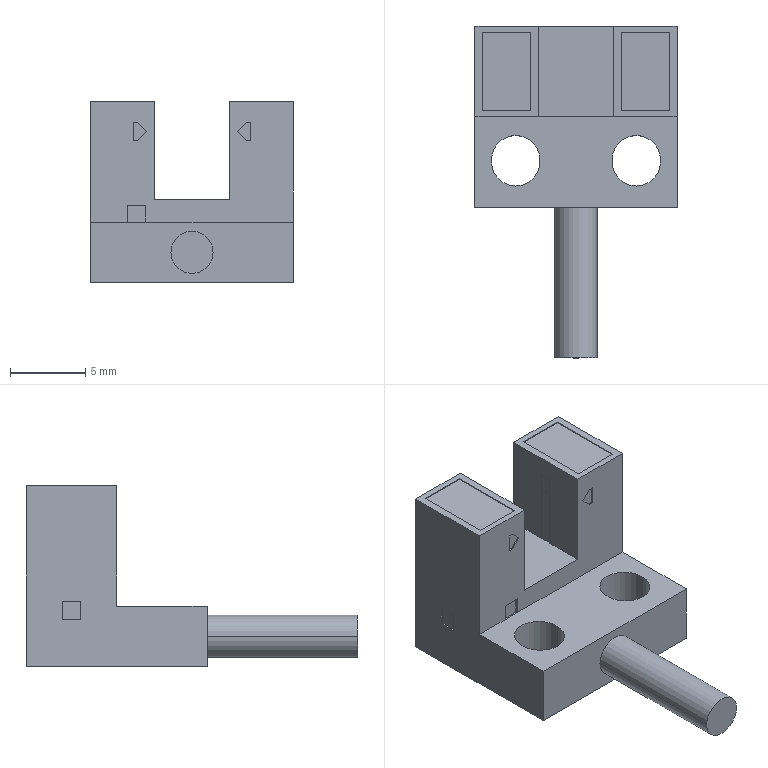Part | SolidWorks | features BaseBody 1 | 1 solid | 87 faces | box 13.4 x 22 x 12 mm | volume 1082 mm3 | plane 79 | cylinder 8 | commonest cylinder face diameters 3.2 x6 2.8 x2